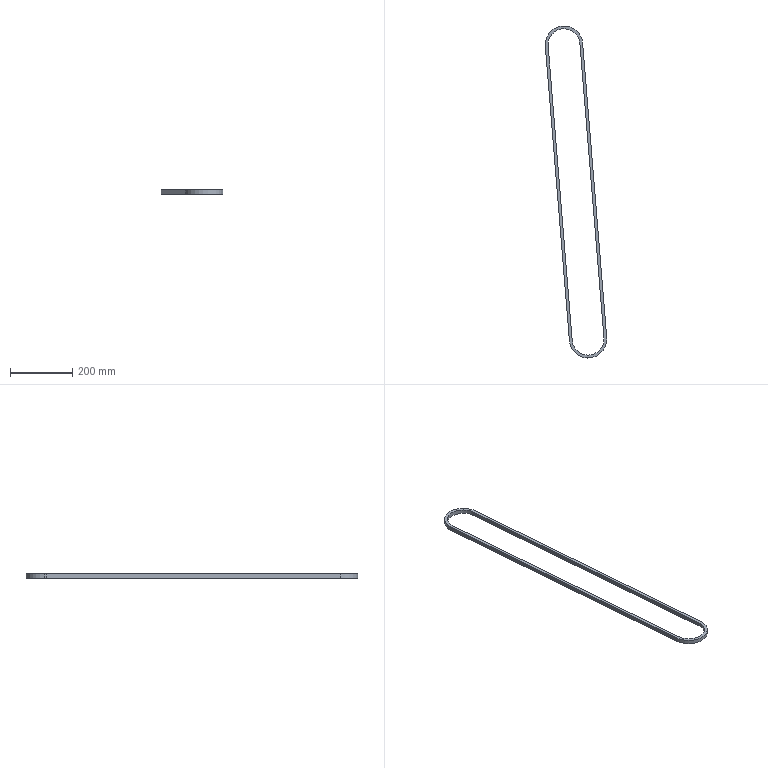Part | STEP file | Pasek_klinowy2V11 | 1 solid | 12 faces | box 197.097 x 1064 x 13 mm | volume 262478 mm3 | cylinder 6 | plane 6 | commonest cylinder face diameters 102 x3 120 x3
STEP:
#1=CARTESIAN_POINT('',(0.,0.,0.));
#2=DIRECTION('',(0.,0.,1.));
#3=DIRECTION('',(1.,0.,0.));
#4=AXIS2_PLACEMENT_3D('',#1,#2,#3);
#5=CARTESIAN_POINT('',(50.831,4.15,13.));
#6=VERTEX_POINT('',#5);
#7=CARTESIAN_POINT('',(50.831,4.15,0.));
#8=VERTEX_POINT('',#7);
#9=CARTESIAN_POINT('',(50.831,4.15,13.));
#10=DIRECTION('',(0.,0.,-1.));
#11=VECTOR('',#10,1.);
#12=LINE('',#9,#11);
#13=CARTESIAN_POINT('',(0.,0.,13.));
#14=DIRECTION('',(0.,0.,-1.));
#15=DIRECTION('',(-1.,0.,0.));
#16=AXIS2_PLACEMENT_3D('',#13,#14,#15);
#17=CYLINDRICAL_SURFACE('',#16,51.);
#18=CARTESIAN_POINT('',(3.06,0.));
#19=DIRECTION('',(0.,1.));
#20=VECTOR('',#19,1.);
#21=LINE('',#18,#20);
#22=(GEOMETRIC_REPRESENTATION_CONTEXT(2)PARAMETRIC_REPRESENTATION_CONTEXT()REPRESENTATION_CONTEXT('',''));
#23=DEFINITIONAL_REPRESENTATION('',(#21),#22);
#24=PCURVE('',#17,#23);
#25=CARTESIAN_POINT('',(50.831,4.15,13.));
#26=DIRECTION('',(-0.9967,-0.08138,0.));
#27=DIRECTION('',(0.08138,-0.9967,0.));
#28=AXIS2_PLACEMENT_3D('',#25,#26,#27);
#29=PLANE('',#28);
#30=CARTESIAN_POINT('',(0.,0.));
#31=DIRECTION('',(0.,-1.));
#32=VECTOR('',#31,1.);
#33=LINE('',#30,#32);
#34=(GEOMETRIC_REPRESENTATION_CONTEXT(2)PARAMETRIC_REPRESENTATION_CONTEXT()REPRESENTATION_CONTEXT('',''));
#35=DEFINITIONAL_REPRESENTATION('',(#33),#34);
#36=PCURVE('',#29,#35);
#37=SURFACE_CURVE('',#12,(#24,#36),.PCURVE_S1.);
#38=EDGE_CURVE('',#6,#8,#37,.T.);
#39=ORIENTED_EDGE('',*,*,#38,.T.);
#40=CARTESIAN_POINT('',(-51.,0.,0.));
#41=VERTEX_POINT('',#40);
#42=CARTESIAN_POINT('',(0.,0.,0.));
#43=DIRECTION('',(0.,0.,1.));
#44=DIRECTION('',(1.,0.,0.));
#45=AXIS2_PLACEMENT_3D('',#42,#43,#44);
#46=CIRCLE('',#45,51.);
#47=CARTESIAN_POINT('',(3.142,13.));
#48=DIRECTION('',(-1.,0.));
#49=VECTOR('',#48,1.);
#50=LINE('',#47,#49);
#51=(GEOMETRIC_REPRESENTATION_CONTEXT(2)PARAMETRIC_REPRESENTATION_CONTEXT()REPRESENTATION_CONTEXT('',''));
#52=DEFINITIONAL_REPRESENTATION('',(#50),#51);
#53=PCURVE('',#17,#52);
#54=CARTESIAN_POINT('',(0.,0.,0.));
#55=DIRECTION('',(0.,0.,1.));
#56=DIRECTION('',(1.,0.,0.));
#57=AXIS2_PLACEMENT_3D('',#54,#55,#56);
#58=PLANE('',#57);
#59=CARTESIAN_POINT('',(0.,0.));
#60=DIRECTION('',(1.,0.));
#61=AXIS2_PLACEMENT_2D('',#59,#60);
#62=CIRCLE('',#61,51.);
#63=(GEOMETRIC_REPRESENTATION_CONTEXT(2)PARAMETRIC_REPRESENTATION_CONTEXT()REPRESENTATION_CONTEXT('',''));
#64=DEFINITIONAL_REPRESENTATION('',(#62),#63);
#65=PCURVE('',#58,#64);
#66=SURFACE_CURVE('',#46,(#53,#65),.PCURVE_S1.);
#67=EDGE_CURVE('',#8,#41,#66,.T.);
#68=ORIENTED_EDGE('',*,*,#67,.T.);
#69=CARTESIAN_POINT('',(-51.,0.,13.));
#70=VERTEX_POINT('',#69);
#71=CARTESIAN_POINT('',(-51.,0.,13.));
#72=DIRECTION('',(0.,0.,-1.));
#73=VECTOR('',#72,1.);
#74=LINE('',#71,#73);
#75=CARTESIAN_POINT('',(0.,0.));
#76=DIRECTION('',(0.,1.));
#77=VECTOR('',#76,1.);
#78=LINE('',#75,#77);
#79=(GEOMETRIC_REPRESENTATION_CONTEXT(2)PARAMETRIC_REPRESENTATION_CONTEXT()REPRESENTATION_CONTEXT('',''));
#80=DEFINITIONAL_REPRESENTATION('',(#78),#79);
#81=PCURVE('',#17,#80);
#82=CARTESIAN_POINT('',(0.,0.,13.));
#83=DIRECTION('',(0.,0.,-1.));
#84=DIRECTION('',(-1.,0.,0.));
#85=AXIS2_PLACEMENT_3D('',#82,#83,#84);
#86=CYLINDRICAL_SURFACE('',#85,51.);
#87=CARTESIAN_POINT('',(6.283,0.));
#88=DIRECTION('',(0.,1.));
#89=VECTOR('',#88,1.);
#90=LINE('',#87,#89);
#91=(GEOMETRIC_REPRESENTATION_CONTEXT(2)PARAMETRIC_REPRESENTATION_CONTEXT()REPRESENTATION_CONTEXT('',''));
#92=DEFINITIONAL_REPRESENTATION('',(#90),#91);
#93=PCURVE('',#86,#92);
#94=SURFACE_CURVE('',#74,(#81,#93),.PCURVE_S1.);
#95=EDGE_CURVE('',#70,#41,#94,.T.);
#96=ORIENTED_EDGE('',*,*,#95,.F.);
#97=CARTESIAN_POINT('',(0.,0.,13.));
#98=DIRECTION('',(0.,0.,1.));
#99=DIRECTION('',(1.,0.,0.));
#100=AXIS2_PLACEMENT_3D('',#97,#98,#99);
#101=CIRCLE('',#100,51.);
#102=CARTESIAN_POINT('',(3.142,0.));
#103=DIRECTION('',(-1.,0.));
#104=VECTOR('',#103,1.);
#105=LINE('',#102,#104);
#106=(GEOMETRIC_REPRESENTATION_CONTEXT(2)PARAMETRIC_REPRESENTATION_CONTEXT()REPRESENTATION_CONTEXT('',''));
#107=DEFINITIONAL_REPRESENTATION('',(#105),#106);
#108=PCURVE('',#17,#107);
#109=CARTESIAN_POINT('',(0.,0.,13.));
#110=DIRECTION('',(0.,0.,1.));
#111=DIRECTION('',(1.,0.,0.));
#112=AXIS2_PLACEMENT_3D('',#109,#110,#111);
#113=PLANE('',#112);
#114=CARTESIAN_POINT('',(0.,0.));
#115=DIRECTION('',(1.,0.));
#116=AXIS2_PLACEMENT_2D('',#114,#115);
#117=CIRCLE('',#116,51.);
#118=(GEOMETRIC_REPRESENTATION_CONTEXT(2)PARAMETRIC_REPRESENTATION_CONTEXT()REPRESENTATION_CONTEXT('',''));
#119=DEFINITIONAL_REPRESENTATION('',(#117),#118);
#120=PCURVE('',#113,#119);
#121=SURFACE_CURVE('',#101,(#108,#120),.PCURVE_S1.);
#122=EDGE_CURVE('',#6,#70,#121,.T.);
#123=ORIENTED_EDGE('',*,*,#122,.F.);
#124=EDGE_LOOP('',(#39,#68,#96,#123));
#125=FACE_BOUND('',#124,.F.);
#126=ADVANCED_FACE('',(#125),#17,.F.);
#127=CARTESIAN_POINT('',(-60.,0.,13.));
#128=VERTEX_POINT('',#127);
#129=CARTESIAN_POINT('',(-59.801,-4.883,13.));
#130=VERTEX_POINT('',#129);
#131=CARTESIAN_POINT('',(0.,0.,13.));
#132=DIRECTION('',(0.,0.,1.));
#133=DIRECTION('',(1.,0.,0.));
#134=AXIS2_PLACEMENT_3D('',#131,#132,#133);
#135=CIRCLE('',#134,60.);
#136=CARTESIAN_POINT('',(0.,0.,13.));
#137=DIRECTION('',(0.,0.,-1.));
#138=DIRECTION('',(-1.,0.,0.));
#139=AXIS2_PLACEMENT_3D('',#136,#137,#138);
#140=CYLINDRICAL_SURFACE('',#139,60.);
#141=CARTESIAN_POINT('',(9.425,0.));
#142=DIRECTION('',(-1.,0.));
#143=VECTOR('',#142,1.);
#144=LINE('',#141,#143);
#145=(GEOMETRIC_REPRESENTATION_CONTEXT(2)PARAMETRIC_REPRESENTATION_CONTEXT()REPRESENTATION_CONTEXT('',''));
#146=DEFINITIONAL_REPRESENTATION('',(#144),#145);
#147=PCURVE('',#140,#146);
#148=CARTESIAN_POINT('',(0.,0.));
#149=DIRECTION('',(1.,0.));
#150=AXIS2_PLACEMENT_2D('',#148,#149);
#151=CIRCLE('',#150,60.);
#152=(GEOMETRIC_REPRESENTATION_CONTEXT(2)PARAMETRIC_REPRESENTATION_CONTEXT()REPRESENTATION_CONTEXT('',''));
#153=DEFINITIONAL_REPRESENTATION('',(#151),#152);
#154=PCURVE('',#113,#153);
#155=SURFACE_CURVE('',#135,(#147,#154),.PCURVE_S1.);
#156=EDGE_CURVE('',#128,#130,#155,.T.);
#157=ORIENTED_EDGE('',*,*,#156,.F.);
#158=CARTESIAN_POINT('',(-60.,0.,0.));
#159=VERTEX_POINT('',#158);
#160=CARTESIAN_POINT('',(-60.,0.,13.));
#161=DIRECTION('',(0.,0.,-1.));
#162=VECTOR('',#161,1.);
#163=LINE('',#160,#162);
#164=CARTESIAN_POINT('',(6.283,0.));
#165=DIRECTION('',(0.,1.));
#166=VECTOR('',#165,1.);
#167=LINE('',#164,#166);
#168=(GEOMETRIC_REPRESENTATION_CONTEXT(2)PARAMETRIC_REPRESENTATION_CONTEXT()REPRESENTATION_CONTEXT('',''));
#169=DEFINITIONAL_REPRESENTATION('',(#167),#168);
#170=PCURVE('',#140,#169);
#171=CARTESIAN_POINT('',(0.,0.,13.));
#172=DIRECTION('',(0.,0.,-1.));
#173=DIRECTION('',(-1.,0.,0.));
#174=AXIS2_PLACEMENT_3D('',#171,#172,#173);
#175=CYLINDRICAL_SURFACE('',#174,60.);
#176=CARTESIAN_POINT('',(0.,0.));
#177=DIRECTION('',(0.,1.));
#178=VECTOR('',#177,1.);
#179=LINE('',#176,#178);
#180=(GEOMETRIC_REPRESENTATION_CONTEXT(2)PARAMETRIC_REPRESENTATION_CONTEXT()REPRESENTATION_CONTEXT('',''));
#181=DEFINITIONAL_REPRESENTATION('',(#179),#180);
#182=PCURVE('',#175,#181);
#183=SURFACE_CURVE('',#163,(#170,#182),.PCURVE_S1.);
#184=EDGE_CURVE('',#128,#159,#183,.T.);
#185=ORIENTED_EDGE('',*,*,#184,.T.);
#186=CARTESIAN_POINT('',(-59.801,-4.883,0.));
#187=VERTEX_POINT('',#186);
#188=CARTESIAN_POINT('',(0.,0.,0.));
#189=DIRECTION('',(0.,0.,1.));
#190=DIRECTION('',(1.,0.,0.));
#191=AXIS2_PLACEMENT_3D('',#188,#189,#190);
#192=CIRCLE('',#191,60.);
#193=CARTESIAN_POINT('',(9.425,13.));
#194=DIRECTION('',(-1.,0.));
#195=VECTOR('',#194,1.);
#196=LINE('',#193,#195);
#197=(GEOMETRIC_REPRESENTATION_CONTEXT(2)PARAMETRIC_REPRESENTATION_CONTEXT()REPRESENTATION_CONTEXT('',''));
#198=DEFINITIONAL_REPRESENTATION('',(#196),#197);
#199=PCURVE('',#140,#198);
#200=CARTESIAN_POINT('',(0.,0.));
#201=DIRECTION('',(1.,0.));
#202=AXIS2_PLACEMENT_2D('',#200,#201);
#203=CIRCLE('',#202,60.);
#204=(GEOMETRIC_REPRESENTATION_CONTEXT(2)PARAMETRIC_REPRESENTATION_CONTEXT()REPRESENTATION_CONTEXT('',''));
#205=DEFINITIONAL_REPRESENTATION('',(#203),#204);
#206=PCURVE('',#58,#205);
#207=SURFACE_CURVE('',#192,(#199,#206),.PCURVE_S1.);
#208=EDGE_CURVE('',#159,#187,#207,.T.);
#209=ORIENTED_EDGE('',*,*,#208,.T.);
#210=CARTESIAN_POINT('',(-59.801,-4.883,13.));
#211=DIRECTION('',(0.,0.,-1.));
#212=VECTOR('',#211,1.);
#213=LINE('',#210,#212);
#214=CARTESIAN_POINT('',(6.202,0.));
#215=DIRECTION('',(0.,1.));
#216=VECTOR('',#215,1.);
#217=LINE('',#214,#216);
#218=(GEOMETRIC_REPRESENTATION_CONTEXT(2)PARAMETRIC_REPRESENTATION_CONTEXT()REPRESENTATION_CONTEXT('',''));
#219=DEFINITIONAL_REPRESENTATION('',(#217),#218);
#220=PCURVE('',#140,#219);
#221=CARTESIAN_POINT('',(-59.801,-4.883,13.));
#222=DIRECTION('',(0.9967,0.08138,0.));
#223=DIRECTION('',(-0.08138,0.9967,0.));
#224=AXIS2_PLACEMENT_3D('',#221,#222,#223);
#225=PLANE('',#224);
#226=CARTESIAN_POINT('',(0.,0.));
#227=DIRECTION('',(0.,-1.));
#228=VECTOR('',#227,1.);
#229=LINE('',#226,#228);
#230=(GEOMETRIC_REPRESENTATION_CONTEXT(2)PARAMETRIC_REPRESENTATION_CONTEXT()REPRESENTATION_CONTEXT('',''));
#231=DEFINITIONAL_REPRESENTATION('',(#229),#230);
#232=PCURVE('',#225,#231);
#233=SURFACE_CURVE('',#213,(#220,#232),.PCURVE_S1.);
#234=EDGE_CURVE('',#130,#187,#233,.T.);
#235=ORIENTED_EDGE('',*,*,#234,.F.);
#236=EDGE_LOOP('',(#157,#185,#209,#235));
#237=FACE_BOUND('',#236,.T.);
#238=ADVANCED_FACE('',(#237),#140,.T.);
#239=CARTESIAN_POINT('',(59.801,4.883,13.));
#240=VERTEX_POINT('',#239);
#241=CARTESIAN_POINT('',(0.,0.,13.));
#242=DIRECTION('',(0.,0.,1.));
#243=DIRECTION('',(1.,0.,0.));
#244=AXIS2_PLACEMENT_3D('',#241,#242,#243);
#245=CIRCLE('',#244,60.);
#246=CARTESIAN_POINT('',(0.,0.));
#247=DIRECTION('',(1.,0.));
#248=AXIS2_PLACEMENT_2D('',#246,#247);
#249=CIRCLE('',#248,60.);
#250=(GEOMETRIC_REPRESENTATION_CONTEXT(2)PARAMETRIC_REPRESENTATION_CONTEXT()REPRESENTATION_CONTEXT('',''));
#251=DEFINITIONAL_REPRESENTATION('',(#249),#250);
#252=PCURVE('',#113,#251);
#253=CARTESIAN_POINT('',(3.142,0.));
#254=DIRECTION('',(-1.,0.));
#255=VECTOR('',#254,1.);
#256=LINE('',#253,#255);
#257=(GEOMETRIC_REPRESENTATION_CONTEXT(2)PARAMETRIC_REPRESENTATION_CONTEXT()REPRESENTATION_CONTEXT('',''));
#258=DEFINITIONAL_REPRESENTATION('',(#256),#257);
#259=PCURVE('',#175,#258);
#260=SURFACE_CURVE('',#245,(#252,#259),.PCURVE_S1.);
#261=EDGE_CURVE('',#240,#128,#260,.T.);
#262=ORIENTED_EDGE('',*,*,#261,.T.);
#263=ORIENTED_EDGE('',*,*,#156,.T.);
#264=CARTESIAN_POINT('',(17.296,-949.083,13.));
#265=VERTEX_POINT('',#264);
#266=CARTESIAN_POINT('',(-59.801,-4.883,13.));
#267=DIRECTION('',(0.08138,-0.9967,0.));
#268=VECTOR('',#267,1.);
#269=LINE('',#266,#268);
#270=CARTESIAN_POINT('',(-59.801,-4.883));
#271=DIRECTION('',(0.08138,-0.9967));
#272=VECTOR('',#271,1.);
#273=LINE('',#270,#272);
#274=(GEOMETRIC_REPRESENTATION_CONTEXT(2)PARAMETRIC_REPRESENTATION_CONTEXT()REPRESENTATION_CONTEXT('',''));
#275=DEFINITIONAL_REPRESENTATION('',(#273),#274);
#276=PCURVE('',#113,#275);
#277=CARTESIAN_POINT('',(0.,0.));
#278=DIRECTION('',(-1.,0.));
#279=VECTOR('',#278,1.);
#280=LINE('',#277,#279);
#281=(GEOMETRIC_REPRESENTATION_CONTEXT(2)PARAMETRIC_REPRESENTATION_CONTEXT()REPRESENTATION_CONTEXT('',''));
#282=DEFINITIONAL_REPRESENTATION('',(#280),#281);
#283=PCURVE('',#225,#282);
#284=SURFACE_CURVE('',#269,(#276,#283),.PCURVE_S1.);
#285=EDGE_CURVE('',#130,#265,#284,.T.);
#286=ORIENTED_EDGE('',*,*,#285,.T.);
#287=CARTESIAN_POINT('',(136.898,-939.317,13.));
#288=VERTEX_POINT('',#287);
#289=CARTESIAN_POINT('',(77.097,-944.2,13.));
#290=DIRECTION('',(0.,0.,1.));
#291=DIRECTION('',(1.,0.,0.));
#292=AXIS2_PLACEMENT_3D('',#289,#290,#291);
#293=CIRCLE('',#292,60.);
#294=CARTESIAN_POINT('',(77.097,-944.2));
#295=DIRECTION('',(1.,0.));
#296=AXIS2_PLACEMENT_2D('',#294,#295);
#297=CIRCLE('',#296,60.);
#298=(GEOMETRIC_REPRESENTATION_CONTEXT(2)PARAMETRIC_REPRESENTATION_CONTEXT()REPRESENTATION_CONTEXT('',''));
#299=DEFINITIONAL_REPRESENTATION('',(#297),#298);
#300=PCURVE('',#113,#299);
#301=CARTESIAN_POINT('',(77.097,-944.2,13.));
#302=DIRECTION('',(0.,0.,-1.));
#303=DIRECTION('',(-1.,0.,0.));
#304=AXIS2_PLACEMENT_3D('',#301,#302,#303);
#305=CYLINDRICAL_SURFACE('',#304,60.);
#306=CARTESIAN_POINT('',(9.425,0.));
#307=DIRECTION('',(-1.,0.));
#308=VECTOR('',#307,1.);
#309=LINE('',#306,#308);
#310=(GEOMETRIC_REPRESENTATION_CONTEXT(2)PARAMETRIC_REPRESENTATION_CONTEXT()REPRESENTATION_CONTEXT('',''));
#311=DEFINITIONAL_REPRESENTATION('',(#309),#310);
#312=PCURVE('',#305,#311);
#313=SURFACE_CURVE('',#293,(#300,#312),.PCURVE_S1.);
#314=EDGE_CURVE('',#265,#288,#313,.T.);
#315=ORIENTED_EDGE('',*,*,#314,.T.);
#316=CARTESIAN_POINT('',(59.801,4.883,13.));
#317=DIRECTION('',(-0.08138,0.9967,0.));
#318=VECTOR('',#317,1.);
#319=LINE('',#316,#318);
#320=CARTESIAN_POINT('',(59.801,4.883));
#321=DIRECTION('',(-0.08138,0.9967));
#322=VECTOR('',#321,1.);
#323=LINE('',#320,#322);
#324=(GEOMETRIC_REPRESENTATION_CONTEXT(2)PARAMETRIC_REPRESENTATION_CONTEXT()REPRESENTATION_CONTEXT('',''));
#325=DEFINITIONAL_REPRESENTATION('',(#323),#324);
#326=PCURVE('',#113,#325);
#327=CARTESIAN_POINT('',(59.801,4.883,13.));
#328=DIRECTION('',(-0.9967,-0.08138,0.));
#329=DIRECTION('',(0.08138,-0.9967,0.));
#330=AXIS2_PLACEMENT_3D('',#327,#328,#329);
#331=PLANE('',#330);
#332=CARTESIAN_POINT('',(0.,0.));
#333=DIRECTION('',(-1.,0.));
#334=VECTOR('',#333,1.);
#335=LINE('',#332,#334);
#336=(GEOMETRIC_REPRESENTATION_CONTEXT(2)PARAMETRIC_REPRESENTATION_CONTEXT()REPRESENTATION_CONTEXT('',''));
#337=DEFINITIONAL_REPRESENTATION('',(#335),#336);
#338=PCURVE('',#331,#337);
#339=SURFACE_CURVE('',#319,(#326,#338),.PCURVE_S1.);
#340=EDGE_CURVE('',#288,#240,#339,.T.);
#341=ORIENTED_EDGE('',*,*,#340,.T.);
#342=EDGE_LOOP('',(#262,#263,#286,#315,#341));
#343=FACE_BOUND('',#342,.T.);
#344=CARTESIAN_POINT('',(-50.831,-4.15,13.));
#345=VERTEX_POINT('',#344);
#346=CARTESIAN_POINT('',(26.266,-948.35,13.));
#347=VERTEX_POINT('',#346);
#348=CARTESIAN_POINT('',(-50.831,-4.15,13.));
#349=DIRECTION('',(0.08138,-0.9967,0.));
#350=VECTOR('',#349,1.);
#351=LINE('',#348,#350);
#352=CARTESIAN_POINT('',(-50.831,-4.15));
#353=DIRECTION('',(0.08138,-0.9967));
#354=VECTOR('',#353,1.);
#355=LINE('',#352,#354);
#356=(GEOMETRIC_REPRESENTATION_CONTEXT(2)PARAMETRIC_REPRESENTATION_CONTEXT()REPRESENTATION_CONTEXT('',''));
#357=DEFINITIONAL_REPRESENTATION('',(#355),#356);
#358=PCURVE('',#113,#357);
#359=CARTESIAN_POINT('',(-50.831,-4.15,13.));
#360=DIRECTION('',(0.9967,0.08138,0.));
#361=DIRECTION('',(-0.08138,0.9967,0.));
#362=AXIS2_PLACEMENT_3D('',#359,#360,#361);
#363=PLANE('',#362);
#364=CARTESIAN_POINT('',(0.,0.));
#365=DIRECTION('',(-1.,0.));
#366=VECTOR('',#365,1.);
#367=LINE('',#364,#366);
#368=(GEOMETRIC_REPRESENTATION_CONTEXT(2)PARAMETRIC_REPRESENTATION_CONTEXT()REPRESENTATION_CONTEXT('',''));
#369=DEFINITIONAL_REPRESENTATION('',(#367),#368);
#370=PCURVE('',#363,#369);
#371=SURFACE_CURVE('',#351,(#358,#370),.PCURVE_S1.);
#372=EDGE_CURVE('',#345,#347,#371,.T.);
#373=ORIENTED_EDGE('',*,*,#372,.F.);
#374=CARTESIAN_POINT('',(0.,0.,13.));
#375=DIRECTION('',(0.,0.,1.));
#376=DIRECTION('',(1.,0.,0.));
#377=AXIS2_PLACEMENT_3D('',#374,#375,#376);
#378=CIRCLE('',#377,51.);
#379=CARTESIAN_POINT('',(0.,0.));
#380=DIRECTION('',(1.,0.));
#381=AXIS2_PLACEMENT_2D('',#379,#380);
#382=CIRCLE('',#381,51.);
#383=(GEOMETRIC_REPRESENTATION_CONTEXT(2)PARAMETRIC_REPRESENTATION_CONTEXT()REPRESENTATION_CONTEXT('',''));
#384=DEFINITIONAL_REPRESENTATION('',(#382),#383);
#385=PCURVE('',#113,#384);
#386=CARTESIAN_POINT('',(9.425,0.));
#387=DIRECTION('',(-1.,0.));
#388=VECTOR('',#387,1.);
#389=LINE('',#386,#388);
#390=(GEOMETRIC_REPRESENTATION_CONTEXT(2)PARAMETRIC_REPRESENTATION_CONTEXT()REPRESENTATION_CONTEXT('',''));
#391=DEFINITIONAL_REPRESENTATION('',(#389),#390);
#392=PCURVE('',#86,#391);
#393=SURFACE_CURVE('',#378,(#385,#392),.PCURVE_S1.);
#394=EDGE_CURVE('',#70,#345,#393,.T.);
#395=ORIENTED_EDGE('',*,*,#394,.F.);
#396=ORIENTED_EDGE('',*,*,#122,.F.);
#397=CARTESIAN_POINT('',(127.928,-940.05,13.));
#398=VERTEX_POINT('',#397);
#399=CARTESIAN_POINT('',(50.831,4.15,13.));
#400=DIRECTION('',(-0.08138,0.9967,0.));
#401=VECTOR('',#400,1.);
#402=LINE('',#399,#401);
#403=CARTESIAN_POINT('',(50.831,4.15));
#404=DIRECTION('',(-0.08138,0.9967));
#405=VECTOR('',#404,1.);
#406=LINE('',#403,#405);
#407=(GEOMETRIC_REPRESENTATION_CONTEXT(2)PARAMETRIC_REPRESENTATION_CONTEXT()REPRESENTATION_CONTEXT('',''));
#408=DEFINITIONAL_REPRESENTATION('',(#406),#407);
#409=PCURVE('',#113,#408);
#410=CARTESIAN_POINT('',(0.,0.));
#411=DIRECTION('',(-1.,0.));
#412=VECTOR('',#411,1.);
#413=LINE('',#410,#412);
#414=(GEOMETRIC_REPRESENTATION_CONTEXT(2)PARAMETRIC_REPRESENTATION_CONTEXT()REPRESENTATION_CONTEXT('',''));
#415=DEFINITIONAL_REPRESENTATION('',(#413),#414);
#416=PCURVE('',#29,#415);
#417=SURFACE_CURVE('',#402,(#409,#416),.PCURVE_S1.);
#418=EDGE_CURVE('',#398,#6,#417,.T.);
#419=ORIENTED_EDGE('',*,*,#418,.F.);
#420=CARTESIAN_POINT('',(77.097,-944.2,13.));
#421=DIRECTION('',(0.,0.,1.));
#422=DIRECTION('',(1.,0.,0.));
#423=AXIS2_PLACEMENT_3D('',#420,#421,#422);
#424=CIRCLE('',#423,51.);
#425=CARTESIAN_POINT('',(77.097,-944.2));
#426=DIRECTION('',(1.,0.));
#427=AXIS2_PLACEMENT_2D('',#425,#426);
#428=CIRCLE('',#427,51.);
#429=(GEOMETRIC_REPRESENTATION_CONTEXT(2)PARAMETRIC_REPRESENTATION_CONTEXT()REPRESENTATION_CONTEXT('',''));
#430=DEFINITIONAL_REPRESENTATION('',(#428),#429);
#431=PCURVE('',#113,#430);
#432=CARTESIAN_POINT('',(77.097,-944.2,13.));
#433=DIRECTION('',(0.,0.,-1.));
#434=DIRECTION('',(-1.,0.,0.));
#435=AXIS2_PLACEMENT_3D('',#432,#433,#434);
#436=CYLINDRICAL_SURFACE('',#435,51.);
#437=CARTESIAN_POINT('',(9.425,0.));
#438=DIRECTION('',(-1.,0.));
#439=VECTOR('',#438,1.);
#440=LINE('',#437,#439);
#441=(GEOMETRIC_REPRESENTATION_CONTEXT(2)PARAMETRIC_REPRESENTATION_CONTEXT()REPRESENTATION_CONTEXT('',''));
#442=DEFINITIONAL_REPRESENTATION('',(#440),#441);
#443=PCURVE('',#436,#442);
#444=SURFACE_CURVE('',#424,(#431,#443),.PCURVE_S1.);
#445=EDGE_CURVE('',#347,#398,#444,.T.);
#446=ORIENTED_EDGE('',*,*,#445,.F.);
#447=EDGE_LOOP('',(#373,#395,#396,#419,#446));
#448=FACE_BOUND('',#447,.T.);
#449=ADVANCED_FACE('',(#343,#448),#113,.T.);
#450=CARTESIAN_POINT('',(59.801,4.883,0.));
#451=VERTEX_POINT('',#450);
#452=CARTESIAN_POINT('',(0.,0.,0.));
#453=DIRECTION('',(0.,0.,1.));
#454=DIRECTION('',(1.,0.,0.));
#455=AXIS2_PLACEMENT_3D('',#452,#453,#454);
#456=CIRCLE('',#455,60.);
#457=CARTESIAN_POINT('',(0.,0.));
#458=DIRECTION('',(1.,0.));
#459=AXIS2_PLACEMENT_2D('',#457,#458);
#460=CIRCLE('',#459,60.);
#461=(GEOMETRIC_REPRESENTATION_CONTEXT(2)PARAMETRIC_REPRESENTATION_CONTEXT()REPRESENTATION_CONTEXT('',''));
#462=DEFINITIONAL_REPRESENTATION('',(#460),#461);
#463=PCURVE('',#58,#462);
#464=CARTESIAN_POINT('',(3.142,13.));
#465=DIRECTION('',(-1.,0.));
#466=VECTOR('',#465,1.);
#467=LINE('',#464,#466);
#468=(GEOMETRIC_REPRESENTATION_CONTEXT(2)PARAMETRIC_REPRESENTATION_CONTEXT()REPRESENTATION_CONTEXT('',''));
#469=DEFINITIONAL_REPRESENTATION('',(#467),#468);
#470=PCURVE('',#175,#469);
#471=SURFACE_CURVE('',#456,(#463,#470),.PCURVE_S1.);
#472=EDGE_CURVE('',#451,#159,#471,.T.);
#473=ORIENTED_EDGE('',*,*,#472,.F.);
#474=CARTESIAN_POINT('',(136.898,-939.317,0.));
#475=VERTEX_POINT('',#474);
#476=CARTESIAN_POINT('',(59.801,4.883,0.));
#477=DIRECTION('',(-0.08138,0.9967,0.));
#478=VECTOR('',#477,1.);
#479=LINE('',#476,#478);
#480=CARTESIAN_POINT('',(59.801,4.883));
#481=DIRECTION('',(-0.08138,0.9967));
#482=VECTOR('',#481,1.);
#483=LINE('',#480,#482);
#484=(GEOMETRIC_REPRESENTATION_CONTEXT(2)PARAMETRIC_REPRESENTATION_CONTEXT()REPRESENTATION_CONTEXT('',''));
#485=DEFINITIONAL_REPRESENTATION('',(#483),#484);
#486=PCURVE('',#58,#485);
#487=CARTESIAN_POINT('',(0.,-13.));
#488=DIRECTION('',(-1.,0.));
#489=VECTOR('',#488,1.);
#490=LINE('',#487,#489);
#491=(GEOMETRIC_REPRESENTATION_CONTEXT(2)PARAMETRIC_REPRESENTATION_CONTEXT()REPRESENTATION_CONTEXT('',''));
#492=DEFINITIONAL_REPRESENTATION('',(#490),#491);
#493=PCURVE('',#331,#492);
#494=SURFACE_CURVE('',#479,(#486,#493),.PCURVE_S1.);
#495=EDGE_CURVE('',#475,#451,#494,.T.);
#496=ORIENTED_EDGE('',*,*,#495,.F.);
#497=CARTESIAN_POINT('',(17.296,-949.083,0.));
#498=VERTEX_POINT('',#497);
#499=CARTESIAN_POINT('',(77.097,-944.2,0.));
#500=DIRECTION('',(0.,0.,1.));
#501=DIRECTION('',(1.,0.,0.));
#502=AXIS2_PLACEMENT_3D('',#499,#500,#501);
#503=CIRCLE('',#502,60.);
#504=CARTESIAN_POINT('',(77.097,-944.2));
#505=DIRECTION('',(1.,0.));
#506=AXIS2_PLACEMENT_2D('',#504,#505);
#507=CIRCLE('',#506,60.);
#508=(GEOMETRIC_REPRESENTATION_CONTEXT(2)PARAMETRIC_REPRESENTATION_CONTEXT()REPRESENTATION_CONTEXT('',''));
#509=DEFINITIONAL_REPRESENTATION('',(#507),#508);
#510=PCURVE('',#58,#509);
#511=CARTESIAN_POINT('',(9.425,13.));
#512=DIRECTION('',(-1.,0.));
#513=VECTOR('',#512,1.);
#514=LINE('',#511,#513);
#515=(GEOMETRIC_REPRESENTATION_CONTEXT(2)PARAMETRIC_REPRESENTATION_CONTEXT()REPRESENTATION_CONTEXT('',''));
#516=DEFINITIONAL_REPRESENTATION('',(#514),#515);
#517=PCURVE('',#305,#516);
#518=SURFACE_CURVE('',#503,(#510,#517),.PCURVE_S1.);
#519=EDGE_CURVE('',#498,#475,#518,.T.);
#520=ORIENTED_EDGE('',*,*,#519,.F.);
#521=CARTESIAN_POINT('',(-59.801,-4.883,0.));
#522=DIRECTION('',(0.08138,-0.9967,0.));
#523=VECTOR('',#522,1.);
#524=LINE('',#521,#523);
#525=CARTESIAN_POINT('',(-59.801,-4.883));
#526=DIRECTION('',(0.08138,-0.9967));
#527=VECTOR('',#526,1.);
#528=LINE('',#525,#527);
#529=(GEOMETRIC_REPRESENTATION_CONTEXT(2)PARAMETRIC_REPRESENTATION_CONTEXT()REPRESENTATION_CONTEXT('',''));
#530=DEFINITIONAL_REPRESENTATION('',(#528),#529);
#531=PCURVE('',#58,#530);
#532=CARTESIAN_POINT('',(0.,-13.));
#533=DIRECTION('',(-1.,0.));
#534=VECTOR('',#533,1.);
#535=LINE('',#532,#534);
#536=(GEOMETRIC_REPRESENTATION_CONTEXT(2)PARAMETRIC_REPRESENTATION_CONTEXT()REPRESENTATION_CONTEXT('',''));
#537=DEFINITIONAL_REPRESENTATION('',(#535),#536);
#538=PCURVE('',#225,#537);
#539=SURFACE_CURVE('',#524,(#531,#538),.PCURVE_S1.);
#540=EDGE_CURVE('',#187,#498,#539,.T.);
#541=ORIENTED_EDGE('',*,*,#540,.F.);
#542=ORIENTED_EDGE('',*,*,#208,.F.);
#543=EDGE_LOOP('',(#473,#496,#520,#541,#542));
#544=FACE_BOUND('',#543,.T.);
#545=ORIENTED_EDGE('',*,*,#67,.T.);
#546=CARTESIAN_POINT('',(-50.831,-4.15,0.));
#547=VERTEX_POINT('',#546);
#548=CARTESIAN_POINT('',(0.,0.,0.));
#549=DIRECTION('',(0.,0.,1.));
#550=DIRECTION('',(1.,0.,0.));
#551=AXIS2_PLACEMENT_3D('',#548,#549,#550);
#552=CIRCLE('',#551,51.);
#553=CARTESIAN_POINT('',(0.,0.));
#554=DIRECTION('',(1.,0.));
#555=AXIS2_PLACEMENT_2D('',#553,#554);
#556=CIRCLE('',#555,51.);
#557=(GEOMETRIC_REPRESENTATION_CONTEXT(2)PARAMETRIC_REPRESENTATION_CONTEXT()REPRESENTATION_CONTEXT('',''));
#558=DEFINITIONAL_REPRESENTATION('',(#556),#557);
#559=PCURVE('',#58,#558);
#560=CARTESIAN_POINT('',(9.425,13.));
#561=DIRECTION('',(-1.,0.));
#562=VECTOR('',#561,1.);
#563=LINE('',#560,#562);
#564=(GEOMETRIC_REPRESENTATION_CONTEXT(2)PARAMETRIC_REPRESENTATION_CONTEXT()REPRESENTATION_CONTEXT('',''));
#565=DEFINITIONAL_REPRESENTATION('',(#563),#564);
#566=PCURVE('',#86,#565);
#567=SURFACE_CURVE('',#552,(#559,#566),.PCURVE_S1.);
#568=EDGE_CURVE('',#41,#547,#567,.T.);
#569=ORIENTED_EDGE('',*,*,#568,.T.);
#570=CARTESIAN_POINT('',(26.266,-948.35,0.));
#571=VERTEX_POINT('',#570);
#572=CARTESIAN_POINT('',(-50.831,-4.15,0.));
#573=DIRECTION('',(0.08138,-0.9967,0.));
#574=VECTOR('',#573,1.);
#575=LINE('',#572,#574);
#576=CARTESIAN_POINT('',(-50.831,-4.15));
#577=DIRECTION('',(0.08138,-0.9967));
#578=VECTOR('',#577,1.);
#579=LINE('',#576,#578);
#580=(GEOMETRIC_REPRESENTATION_CONTEXT(2)PARAMETRIC_REPRESENTATION_CONTEXT()REPRESENTATION_CONTEXT('',''));
#581=DEFINITIONAL_REPRESENTATION('',(#579),#580);
#582=PCURVE('',#58,#581);
#583=CARTESIAN_POINT('',(0.,-13.));
#584=DIRECTION('',(-1.,0.));
#585=VECTOR('',#584,1.);
#586=LINE('',#583,#585);
#587=(GEOMETRIC_REPRESENTATION_CONTEXT(2)PARAMETRIC_REPRESENTATION_CONTEXT()REPRESENTATION_CONTEXT('',''));
#588=DEFINITIONAL_REPRESENTATION('',(#586),#587);
#589=PCURVE('',#363,#588);
#590=SURFACE_CURVE('',#575,(#582,#589),.PCURVE_S1.);
#591=EDGE_CURVE('',#547,#571,#590,.T.);
#592=ORIENTED_EDGE('',*,*,#591,.T.);
#593=CARTESIAN_POINT('',(127.928,-940.05,0.));
#594=VERTEX_POINT('',#593);
#595=CARTESIAN_POINT('',(77.097,-944.2,0.));
#596=DIRECTION('',(0.,0.,1.));
#597=DIRECTION('',(1.,0.,0.));
#598=AXIS2_PLACEMENT_3D('',#595,#596,#597);
#599=CIRCLE('',#598,51.);
#600=CARTESIAN_POINT('',(77.097,-944.2));
#601=DIRECTION('',(1.,0.));
#602=AXIS2_PLACEMENT_2D('',#600,#601);
#603=CIRCLE('',#602,51.);
#604=(GEOMETRIC_REPRESENTATION_CONTEXT(2)PARAMETRIC_REPRESENTATION_CONTEXT()REPRESENTATION_CONTEXT('',''));
#605=DEFINITIONAL_REPRESENTATION('',(#603),#604);
#606=PCURVE('',#58,#605);
#607=CARTESIAN_POINT('',(9.425,13.));
#608=DIRECTION('',(-1.,0.));
#609=VECTOR('',#608,1.);
#610=LINE('',#607,#609);
#611=(GEOMETRIC_REPRESENTATION_CONTEXT(2)PARAMETRIC_REPRESENTATION_CONTEXT()REPRESENTATION_CONTEXT('',''));
#612=DEFINITIONAL_REPRESENTATION('',(#610),#611);
#613=PCURVE('',#436,#612);
#614=SURFACE_CURVE('',#599,(#606,#613),.PCURVE_S1.);
#615=EDGE_CURVE('',#571,#594,#614,.T.);
#616=ORIENTED_EDGE('',*,*,#615,.T.);
#617=CARTESIAN_POINT('',(50.831,4.15,0.));
#618=DIRECTION('',(-0.08138,0.9967,0.));
#619=VECTOR('',#618,1.);
#620=LINE('',#617,#619);
#621=CARTESIAN_POINT('',(50.831,4.15));
#622=DIRECTION('',(-0.08138,0.9967));
#623=VECTOR('',#622,1.);
#624=LINE('',#621,#623);
#625=(GEOMETRIC_REPRESENTATION_CONTEXT(2)PARAMETRIC_REPRESENTATION_CONTEXT()REPRESENTATION_CONTEXT('',''));
#626=DEFINITIONAL_REPRESENTATION('',(#624),#625);
#627=PCURVE('',#58,#626);
#628=CARTESIAN_POINT('',(0.,-13.));
#629=DIRECTION('',(-1.,0.));
#630=VECTOR('',#629,1.);
#631=LINE('',#628,#630);
#632=(GEOMETRIC_REPRESENTATION_CONTEXT(2)PARAMETRIC_REPRESENTATION_CONTEXT()REPRESENTATION_CONTEXT('',''));
#633=DEFINITIONAL_REPRESENTATION('',(#631),#632);
#634=PCURVE('',#29,#633);
#635=SURFACE_CURVE('',#620,(#627,#634),.PCURVE_S1.);
#636=EDGE_CURVE('',#594,#8,#635,.T.);
#637=ORIENTED_EDGE('',*,*,#636,.T.);
#638=EDGE_LOOP('',(#545,#569,#592,#616,#637));
#639=FACE_BOUND('',#638,.T.);
#640=ADVANCED_FACE('',(#544,#639),#58,.F.);
#641=ORIENTED_EDGE('',*,*,#184,.F.);
#642=ORIENTED_EDGE('',*,*,#261,.F.);
#643=CARTESIAN_POINT('',(59.801,4.883,13.));
#644=DIRECTION('',(0.,0.,-1.));
#645=VECTOR('',#644,1.);
#646=LINE('',#643,#645);
#647=CARTESIAN_POINT('',(3.06,0.));
#648=DIRECTION('',(0.,1.));
#649=VECTOR('',#648,1.);
#650=LINE('',#647,#649);
#651=(GEOMETRIC_REPRESENTATION_CONTEXT(2)PARAMETRIC_REPRESENTATION_CONTEXT()REPRESENTATION_CONTEXT('',''));
#652=DEFINITIONAL_REPRESENTATION('',(#650),#651);
#653=PCURVE('',#175,#652);
#654=CARTESIAN_POINT('',(0.,0.));
#655=DIRECTION('',(0.,-1.));
#656=VECTOR('',#655,1.);
#657=LINE('',#654,#656);
#658=(GEOMETRIC_REPRESENTATION_CONTEXT(2)PARAMETRIC_REPRESENTATION_CONTEXT()REPRESENTATION_CONTEXT('',''));
#659=DEFINITIONAL_REPRESENTATION('',(#657),#658);
#660=PCURVE('',#331,#659);
#661=SURFACE_CURVE('',#646,(#653,#660),.PCURVE_S1.);
#662=EDGE_CURVE('',#240,#451,#661,.T.);
#663=ORIENTED_EDGE('',*,*,#662,.T.);
#664=ORIENTED_EDGE('',*,*,#472,.T.);
#665=EDGE_LOOP('',(#641,#642,#663,#664));
#666=FACE_BOUND('',#665,.T.);
#667=ADVANCED_FACE('',(#666),#175,.T.);
#668=ORIENTED_EDGE('',*,*,#540,.T.);
#669=CARTESIAN_POINT('',(17.296,-949.083,13.));
#670=DIRECTION('',(0.,0.,-1.));
#671=VECTOR('',#670,1.);
#672=LINE('',#669,#671);
#673=CARTESIAN_POINT('',(-947.342,0.));
#674=DIRECTION('',(0.,-1.));
#675=VECTOR('',#674,1.);
#676=LINE('',#673,#675);
#677=(GEOMETRIC_REPRESENTATION_CONTEXT(2)PARAMETRIC_REPRESENTATION_CONTEXT()REPRESENTATION_CONTEXT('',''));
#678=DEFINITIONAL_REPRESENTATION('',(#676),#677);
#679=PCURVE('',#225,#678);
#680=CARTESIAN_POINT('',(6.202,0.));
#681=DIRECTION('',(0.,1.));
#682=VECTOR('',#681,1.);
#683=LINE('',#680,#682);
#684=(GEOMETRIC_REPRESENTATION_CONTEXT(2)PARAMETRIC_REPRESENTATION_CONTEXT()REPRESENTATION_CONTEXT('',''));
#685=DEFINITIONAL_REPRESENTATION('',(#683),#684);
#686=PCURVE('',#305,#685);
#687=SURFACE_CURVE('',#672,(#679,#686),.PCURVE_S1.);
#688=EDGE_CURVE('',#265,#498,#687,.T.);
#689=ORIENTED_EDGE('',*,*,#688,.F.);
#690=ORIENTED_EDGE('',*,*,#285,.F.);
#691=ORIENTED_EDGE('',*,*,#234,.T.);
#692=EDGE_LOOP('',(#668,#689,#690,#691));
#693=FACE_BOUND('',#692,.T.);
#694=ADVANCED_FACE('',(#693),#225,.F.);
#695=ORIENTED_EDGE('',*,*,#519,.T.);
#696=CARTESIAN_POINT('',(136.898,-939.317,13.));
#697=DIRECTION('',(0.,0.,-1.));
#698=VECTOR('',#697,1.);
#699=LINE('',#696,#698);
#700=CARTESIAN_POINT('',(3.06,0.));
#701=DIRECTION('',(0.,1.));
#702=VECTOR('',#701,1.);
#703=LINE('',#700,#702);
#704=(GEOMETRIC_REPRESENTATION_CONTEXT(2)PARAMETRIC_REPRESENTATION_CONTEXT()REPRESENTATION_CONTEXT('',''));
#705=DEFINITIONAL_REPRESENTATION('',(#703),#704);
#706=PCURVE('',#305,#705);
#707=CARTESIAN_POINT('',(947.342,0.));
#708=DIRECTION('',(0.,-1.));
#709=VECTOR('',#708,1.);
#710=LINE('',#707,#709);
#711=(GEOMETRIC_REPRESENTATION_CONTEXT(2)PARAMETRIC_REPRESENTATION_CONTEXT()REPRESENTATION_CONTEXT('',''));
#712=DEFINITIONAL_REPRESENTATION('',(#710),#711);
#713=PCURVE('',#331,#712);
#714=SURFACE_CURVE('',#699,(#706,#713),.PCURVE_S1.);
#715=EDGE_CURVE('',#288,#475,#714,.T.);
#716=ORIENTED_EDGE('',*,*,#715,.F.);
#717=ORIENTED_EDGE('',*,*,#314,.F.);
#718=ORIENTED_EDGE('',*,*,#688,.T.);
#719=EDGE_LOOP('',(#695,#716,#717,#718));
#720=FACE_BOUND('',#719,.T.);
#721=ADVANCED_FACE('',(#720),#305,.T.);
#722=ORIENTED_EDGE('',*,*,#495,.T.);
#723=ORIENTED_EDGE('',*,*,#662,.F.);
#724=ORIENTED_EDGE('',*,*,#340,.F.);
#725=ORIENTED_EDGE('',*,*,#715,.T.);
#726=EDGE_LOOP('',(#722,#723,#724,#725));
#727=FACE_BOUND('',#726,.T.);
#728=ADVANCED_FACE('',(#727),#331,.F.);
#729=ORIENTED_EDGE('',*,*,#568,.T.);
#730=CARTESIAN_POINT('',(-50.831,-4.15,13.));
#731=DIRECTION('',(0.,0.,-1.));
#732=VECTOR('',#731,1.);
#733=LINE('',#730,#732);
#734=CARTESIAN_POINT('',(6.202,0.));
#735=DIRECTION('',(0.,1.));
#736=VECTOR('',#735,1.);
#737=LINE('',#734,#736);
#738=(GEOMETRIC_REPRESENTATION_CONTEXT(2)PARAMETRIC_REPRESENTATION_CONTEXT()REPRESENTATION_CONTEXT('',''));
#739=DEFINITIONAL_REPRESENTATION('',(#737),#738);
#740=PCURVE('',#86,#739);
#741=CARTESIAN_POINT('',(0.,0.));
#742=DIRECTION('',(0.,-1.));
#743=VECTOR('',#742,1.);
#744=LINE('',#741,#743);
#745=(GEOMETRIC_REPRESENTATION_CONTEXT(2)PARAMETRIC_REPRESENTATION_CONTEXT()REPRESENTATION_CONTEXT('',''));
#746=DEFINITIONAL_REPRESENTATION('',(#744),#745);
#747=PCURVE('',#363,#746);
#748=SURFACE_CURVE('',#733,(#740,#747),.PCURVE_S1.);
#749=EDGE_CURVE('',#345,#547,#748,.T.);
#750=ORIENTED_EDGE('',*,*,#749,.F.);
#751=ORIENTED_EDGE('',*,*,#394,.F.);
#752=ORIENTED_EDGE('',*,*,#95,.T.);
#753=EDGE_LOOP('',(#729,#750,#751,#752));
#754=FACE_BOUND('',#753,.F.);
#755=ADVANCED_FACE('',(#754),#86,.F.);
#756=ORIENTED_EDGE('',*,*,#591,.F.);
#757=ORIENTED_EDGE('',*,*,#749,.F.);
#758=ORIENTED_EDGE('',*,*,#372,.T.);
#759=CARTESIAN_POINT('',(26.266,-948.35,13.));
#760=DIRECTION('',(0.,0.,-1.));
#761=VECTOR('',#760,1.);
#762=LINE('',#759,#761);
#763=CARTESIAN_POINT('',(-947.342,0.));
#764=DIRECTION('',(0.,-1.));
#765=VECTOR('',#764,1.);
#766=LINE('',#763,#765);
#767=(GEOMETRIC_REPRESENTATION_CONTEXT(2)PARAMETRIC_REPRESENTATION_CONTEXT()REPRESENTATION_CONTEXT('',''));
#768=DEFINITIONAL_REPRESENTATION('',(#766),#767);
#769=PCURVE('',#363,#768);
#770=CARTESIAN_POINT('',(6.202,0.));
#771=DIRECTION('',(0.,1.));
#772=VECTOR('',#771,1.);
#773=LINE('',#770,#772);
#774=(GEOMETRIC_REPRESENTATION_CONTEXT(2)PARAMETRIC_REPRESENTATION_CONTEXT()REPRESENTATION_CONTEXT('',''));
#775=DEFINITIONAL_REPRESENTATION('',(#773),#774);
#776=PCURVE('',#436,#775);
#777=SURFACE_CURVE('',#762,(#769,#776),.PCURVE_S1.);
#778=EDGE_CURVE('',#347,#571,#777,.T.);
#779=ORIENTED_EDGE('',*,*,#778,.T.);
#780=EDGE_LOOP('',(#756,#757,#758,#779));
#781=FACE_BOUND('',#780,.T.);
#782=ADVANCED_FACE('',(#781),#363,.T.);
#783=CARTESIAN_POINT('',(127.928,-940.05,13.));
#784=DIRECTION('',(0.,0.,-1.));
#785=VECTOR('',#784,1.);
#786=LINE('',#783,#785);
#787=CARTESIAN_POINT('',(3.06,0.));
#788=DIRECTION('',(0.,1.));
#789=VECTOR('',#788,1.);
#790=LINE('',#787,#789);
#791=(GEOMETRIC_REPRESENTATION_CONTEXT(2)PARAMETRIC_REPRESENTATION_CONTEXT()REPRESENTATION_CONTEXT('',''));
#792=DEFINITIONAL_REPRESENTATION('',(#790),#791);
#793=PCURVE('',#436,#792);
#794=CARTESIAN_POINT('',(947.342,0.));
#795=DIRECTION('',(0.,-1.));
#796=VECTOR('',#795,1.);
#797=LINE('',#794,#796);
#798=(GEOMETRIC_REPRESENTATION_CONTEXT(2)PARAMETRIC_REPRESENTATION_CONTEXT()REPRESENTATION_CONTEXT('',''));
#799=DEFINITIONAL_REPRESENTATION('',(#797),#798);
#800=PCURVE('',#29,#799);
#801=SURFACE_CURVE('',#786,(#793,#800),.PCURVE_S1.);
#802=EDGE_CURVE('',#398,#594,#801,.T.);
#803=ORIENTED_EDGE('',*,*,#802,.F.);
#804=ORIENTED_EDGE('',*,*,#445,.F.);
#805=ORIENTED_EDGE('',*,*,#778,.T.);
#806=ORIENTED_EDGE('',*,*,#615,.T.);
#807=EDGE_LOOP('',(#803,#804,#805,#806));
#808=FACE_BOUND('',#807,.F.);
#809=ADVANCED_FACE('',(#808),#436,.F.);
#810=ORIENTED_EDGE('',*,*,#636,.F.);
#811=ORIENTED_EDGE('',*,*,#802,.F.);
#812=ORIENTED_EDGE('',*,*,#418,.T.);
#813=ORIENTED_EDGE('',*,*,#38,.T.);
#814=EDGE_LOOP('',(#810,#811,#812,#813));
#815=FACE_BOUND('',#814,.T.);
#816=ADVANCED_FACE('',(#815),#29,.T.);
#817=CLOSED_SHELL('',(#126,#238,#449,#640,#667,#694,#721,#728,#755,#782,#809,#816));
#818=MANIFOLD_SOLID_BREP('',#817);
#819=(LENGTH_UNIT()NAMED_UNIT(*)SI_UNIT(.MILLI.,.METRE.));
#820=UNCERTAINTY_MEASURE_WITH_UNIT(LENGTH_MEASURE(0.0000001),#819,'','');
#821=(NAMED_UNIT(*)PLANE_ANGLE_UNIT()SI_UNIT($,.RADIAN.));
#822=(NAMED_UNIT(*)SI_UNIT($,.STERADIAN.)SOLID_ANGLE_UNIT());
#823=(GEOMETRIC_REPRESENTATION_CONTEXT(3)GLOBAL_UNCERTAINTY_ASSIGNED_CONTEXT((#820))GLOBAL_UNIT_ASSIGNED_CONTEXT((#819,#821,#822))REPRESENTATION_CONTEXT('',''));
#824=ADVANCED_BREP_SHAPE_REPRESENTATION('',(#4,#818),#823);